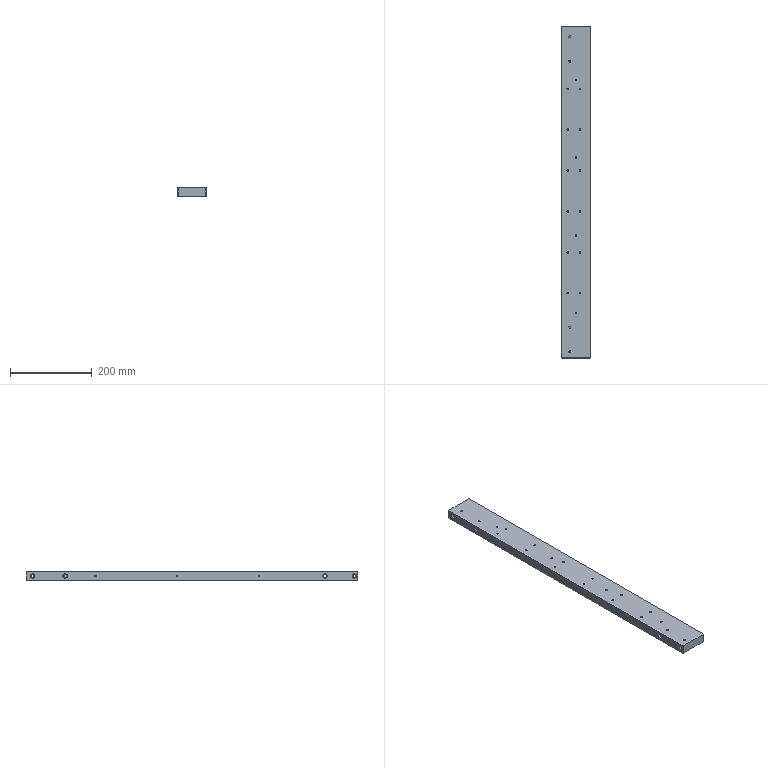Part | NX | features BREP 1 | 1 solid | 90 faces | box 70 x 813 x 22 mm | volume 1233369 mm3 | cylinder 66 | plane 14 | cone 10 | commonest cylinder face diameters 4.2 x32 5 x12 6.6 x8 11 x8 3.3 x6